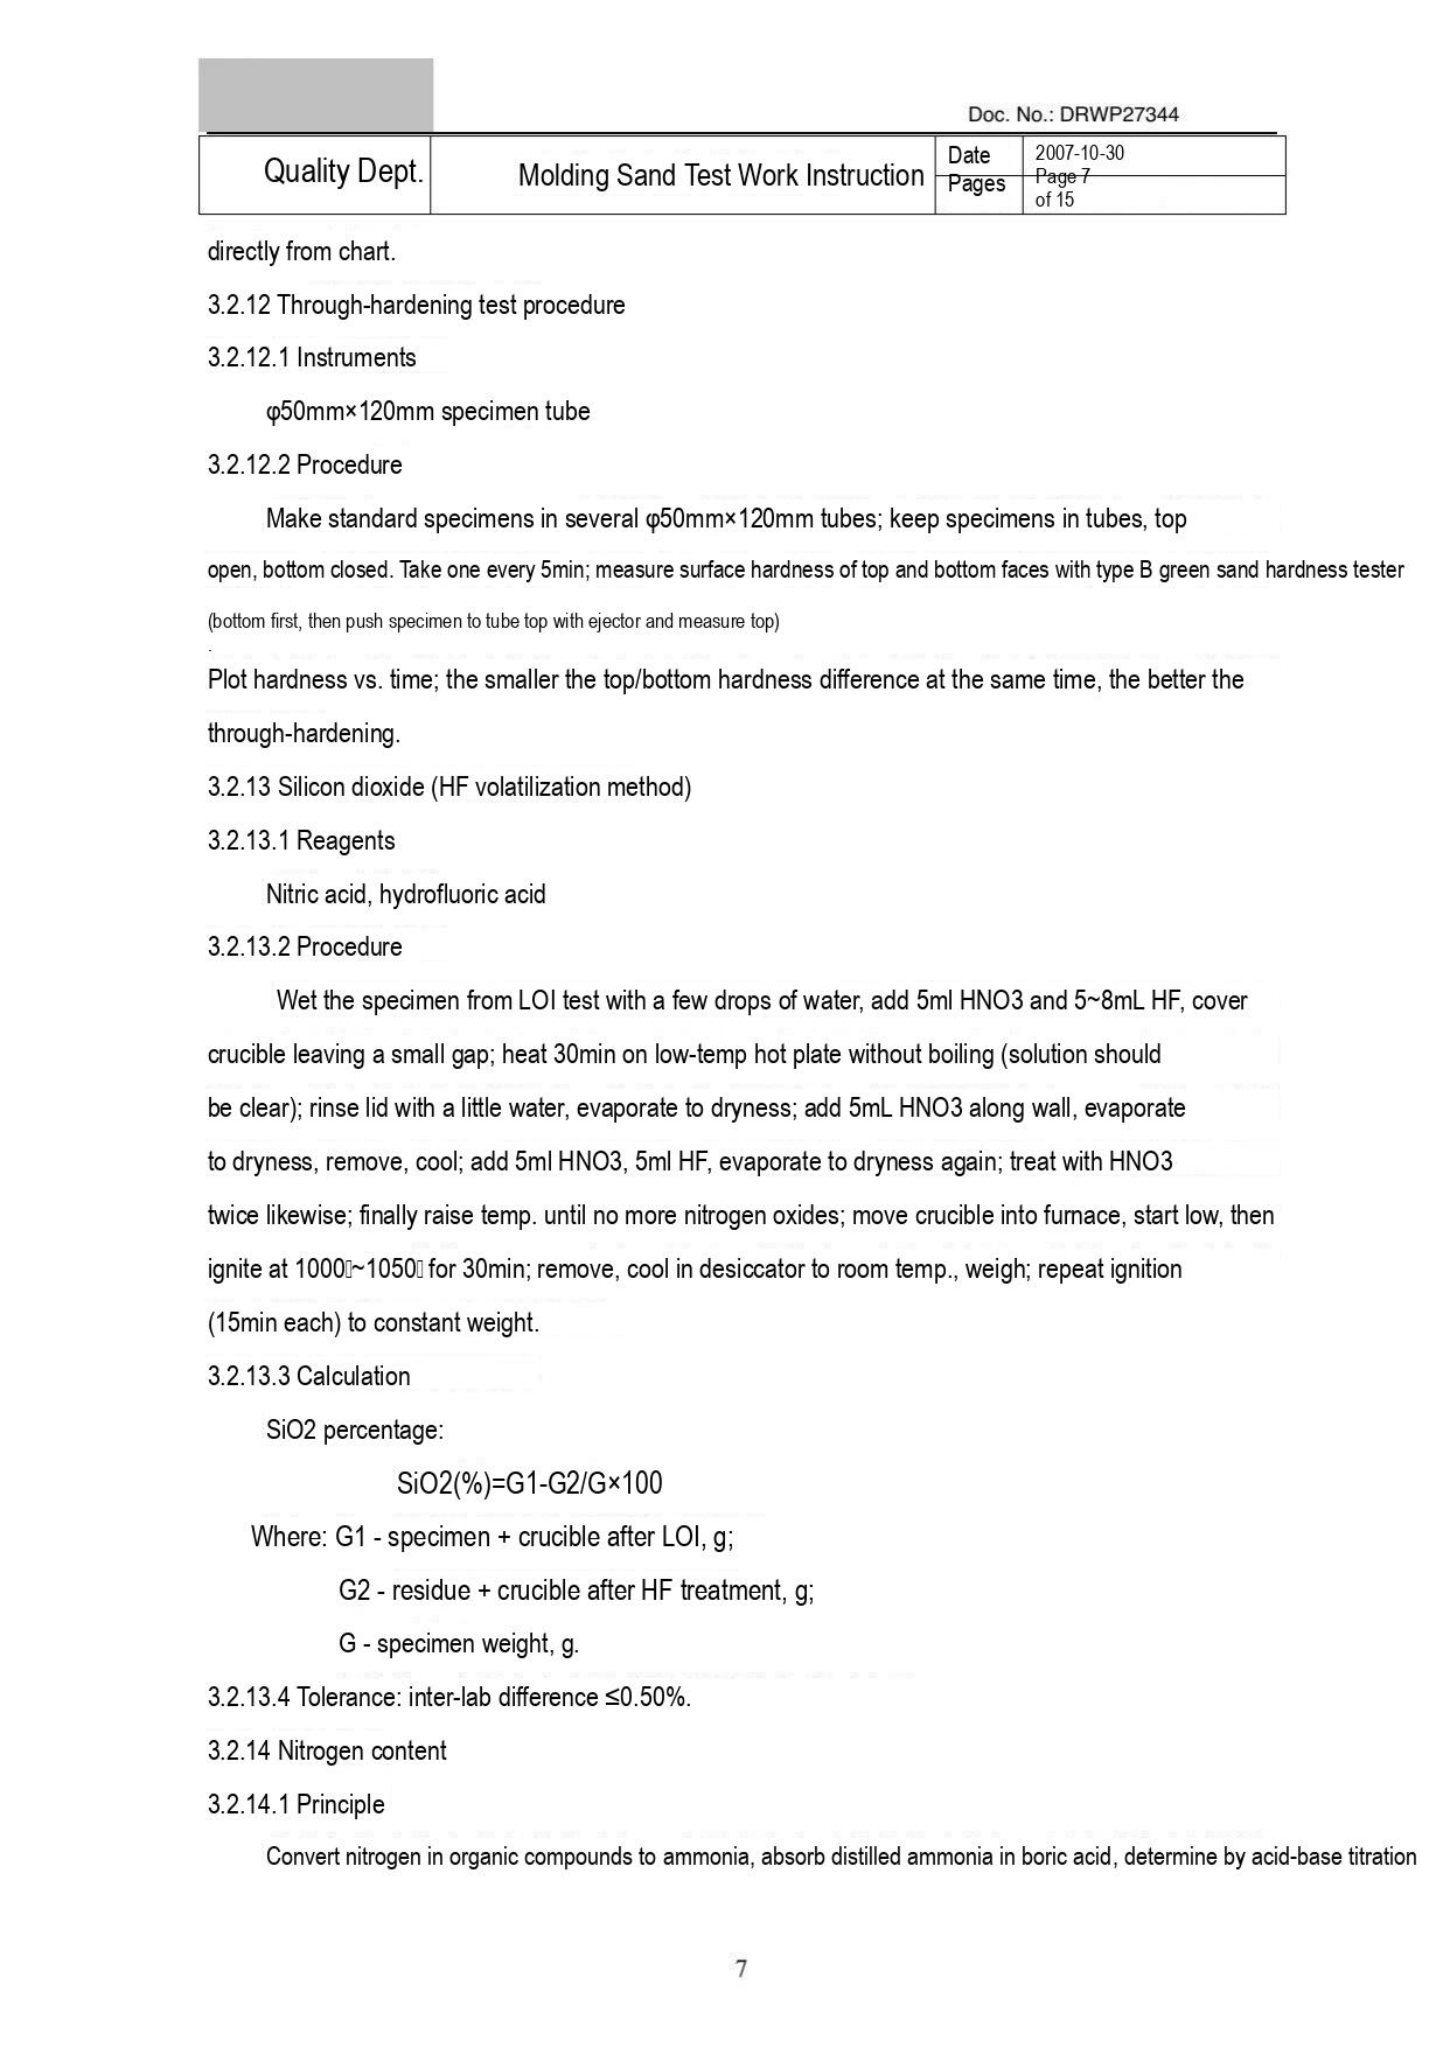Doc. No.: DRWP27344

| Quality Dept. | Molding Sand Test Work Instruction | Date | 2007-10-30 |
|---|---|---|---|
| | | Pages | Page 7 of 15 |

directly from chart.

3.2.12 Through-hardening test procedure

3.2.12.1 Instruments

φ50mm×120mm specimen tube

3.2.12.2 Procedure

Make standard specimens in several φ50mm×120mm tubes; keep specimens in tubes, top open, bottom closed. Take one every 5min; measure surface hardness of top and bottom faces with type B green sand hardness tester (bottom first, then push specimen to tube top with ejector and measure top)

Plot hardness vs. time; the smaller the top/bottom hardness difference at the same time, the better the through-hardening.

3.2.13 Silicon dioxide (HF volatilization method)

3.2.13.1 Reagents

Nitric acid, hydrofluoric acid

3.2.13.2 Procedure

Wet the specimen from LOI test with a few drops of water, add 5ml HNO3 and 5~8mL HF, cover crucible leaving a small gap; heat 30min on low-temp hot plate without boiling (solution should be clear); rinse lid with a little water, evaporate to dryness; add 5mL HNO3 along wall, evaporate to dryness, remove, cool; add 5ml HNO3, 5ml HF, evaporate to dryness again; treat with HNO3 twice likewise; finally raise temp. until no more nitrogen oxides; move crucible into furnace, start low, then ignite at 1000~1050 for 30min; remove, cool in desiccator to room temp., weigh; repeat ignition (15min each) to constant weight.

3.2.13.3 Calculation

SiO2 percentage:

SiO2(%)=G1-G2/G×100

Where: G1 - specimen + crucible after LOI, g;

G2 - residue + crucible after HF treatment, g;

G - specimen weight, g.

3.2.13.4 Tolerance: inter-lab difference ≤0.50%.

3.2.14 Nitrogen content

3.2.14.1 Principle

Convert nitrogen in organic compounds to ammonia, absorb distilled ammonia in boric acid, determine by acid-base titration

7
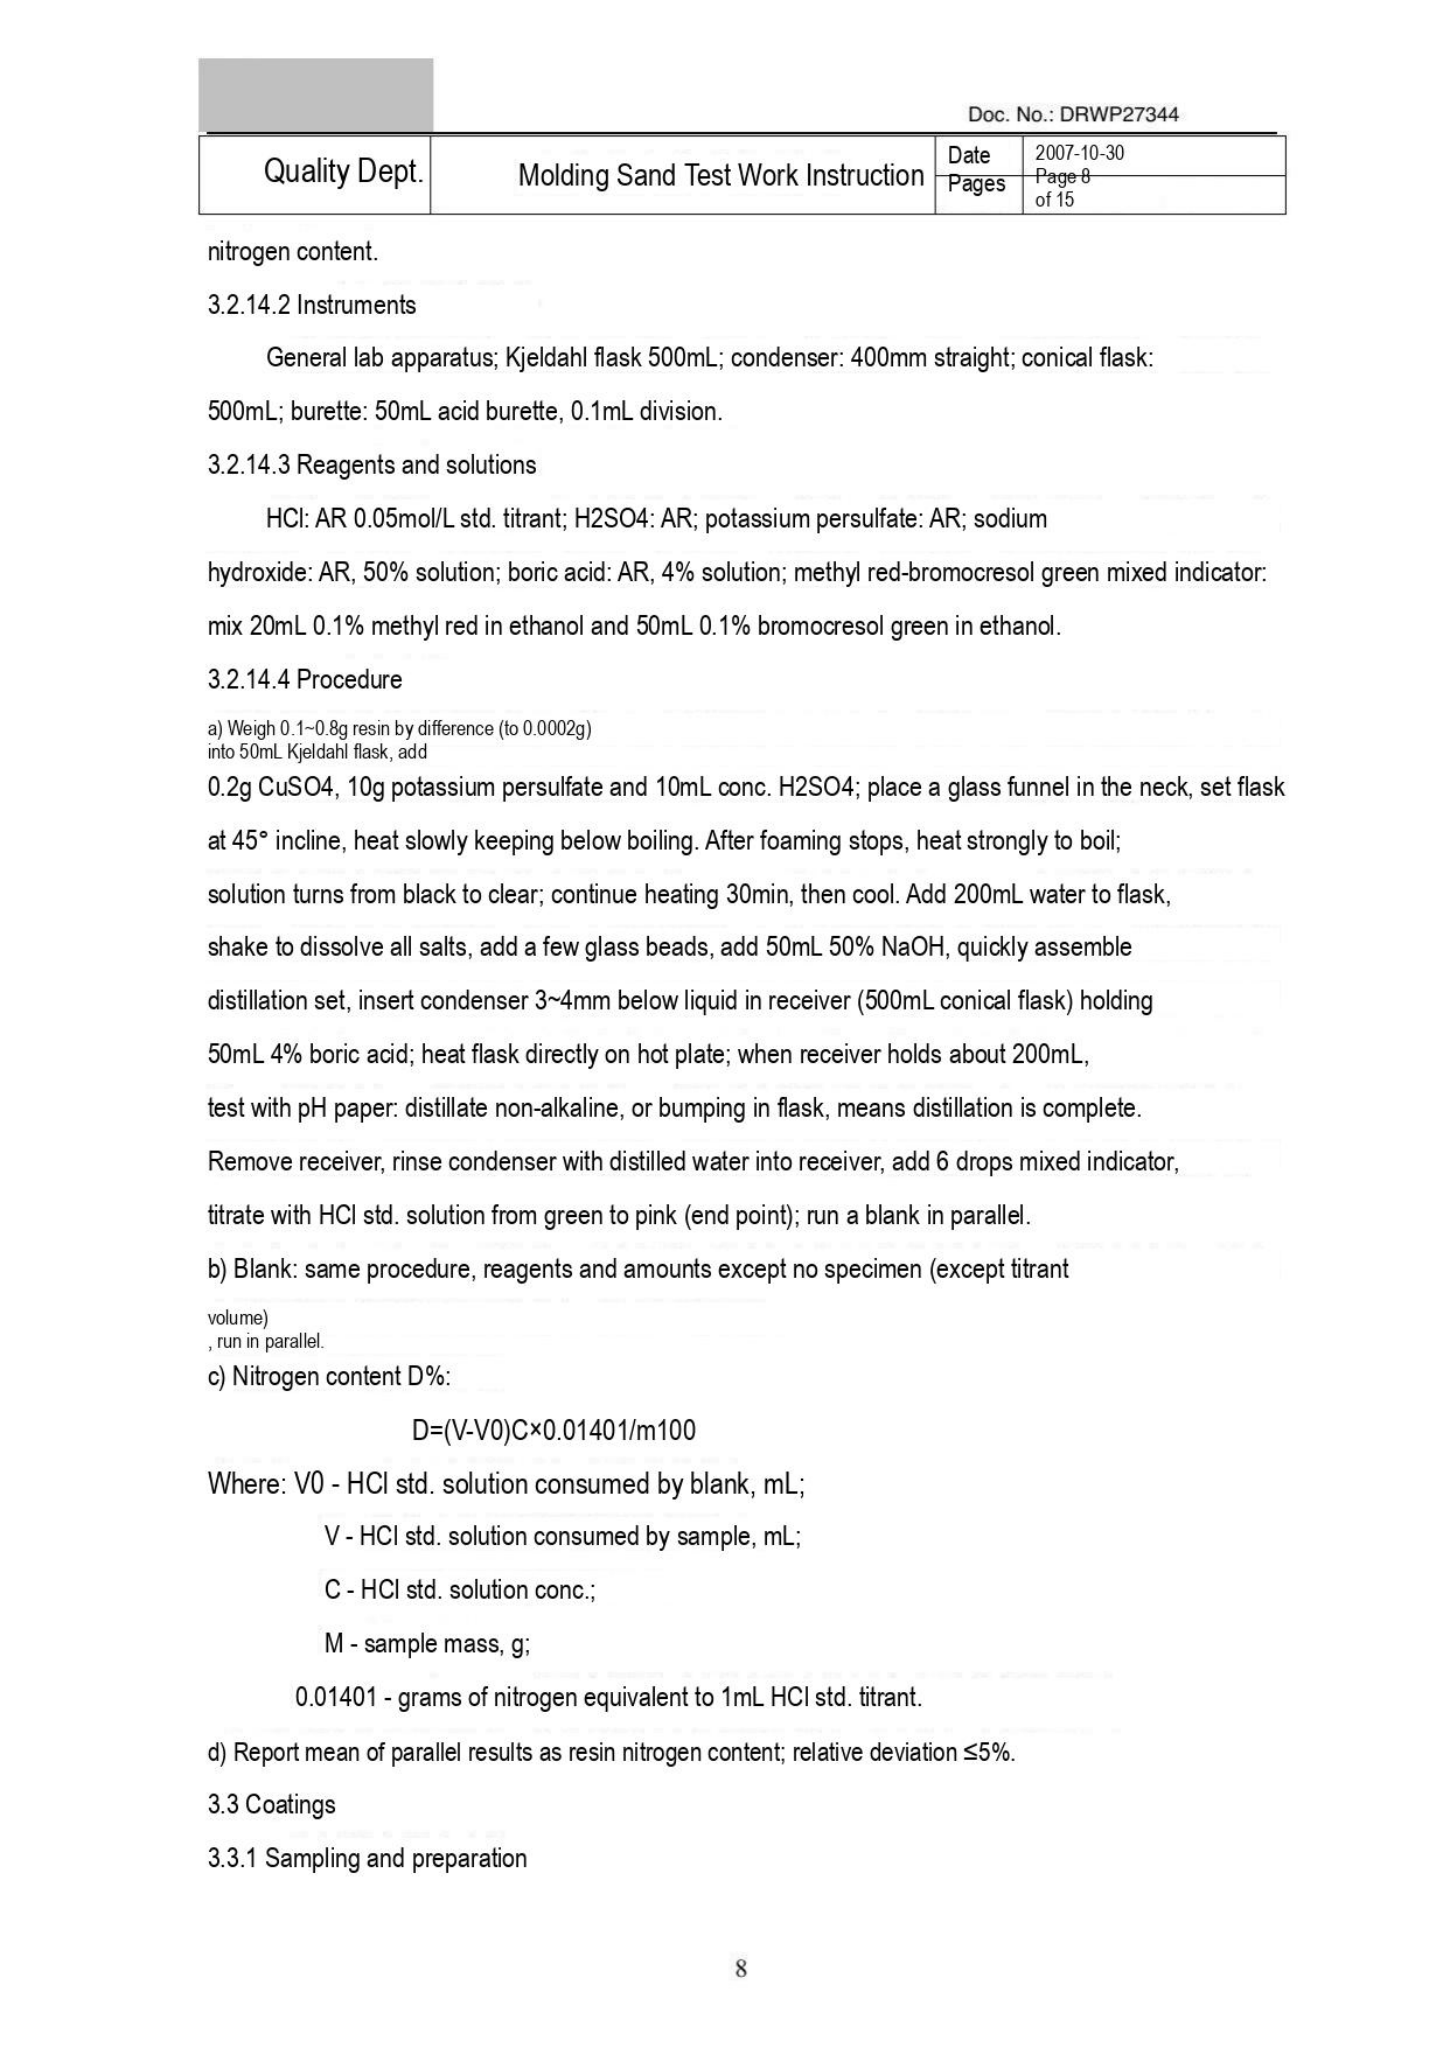Doc. No.: DRWP27344

| Quality Dept. | Molding Sand Test Work Instruction | Date | 2007-10-30 |
|---|---|---|---|
| | | Pages | Page 8 of 15 |

nitrogen content.

3.2.14.2 Instruments

General lab apparatus; Kjeldahl flask 500mL; condenser: 400mm straight; conical flask: 500mL; burette: 50mL acid burette, 0.1mL division.

3.2.14.3 Reagents and solutions

HCl: AR 0.05mol/L std. titrant; H2SO4: AR; potassium persulfate: AR; sodium hydroxide: AR, 50% solution; boric acid: AR, 4% solution; methyl red-bromocresol green mixed indicator: mix 20mL 0.1% methyl red in ethanol and 50mL 0.1% bromocresol green in ethanol.

3.2.14.4 Procedure

a) Weigh 0.1~0.8g resin by difference (to 0.0002g)
into 50mL Kjeldahl flask, add
0.2g CuSO4, 10g potassium persulfate and 10mL conc. H2SO4; place a glass funnel in the neck, set flask at 45° incline, heat slowly keeping below boiling. After foaming stops, heat strongly to boil; solution turns from black to clear; continue heating 30min, then cool. Add 200mL water to flask, shake to dissolve all salts, add a few glass beads, add 50mL 50% NaOH, quickly assemble distillation set, insert condenser 3~4mm below liquid in receiver (500mL conical flask) holding 50mL 4% boric acid; heat flask directly on hot plate; when receiver holds about 200mL, test with pH paper: distillate non-alkaline, or bumping in flask, means distillation is complete. Remove receiver, rinse condenser with distilled water into receiver, add 6 drops mixed indicator, titrate with HCl std. solution from green to pink (end point); run a blank in parallel.

b) Blank: same procedure, reagents and amounts except no specimen (except titrant
volume)
, run in parallel.

c) Nitrogen content D%:

D=(V-V0)C×0.01401/m100

Where: V0 - HCl std. solution consumed by blank, mL;

V - HCl std. solution consumed by sample, mL;

C - HCl std. solution conc.;

M - sample mass, g;

0.01401 - grams of nitrogen equivalent to 1mL HCl std. titrant.

d) Report mean of parallel results as resin nitrogen content; relative deviation ≤5%.

3.3 Coatings

3.3.1 Sampling and preparation

8
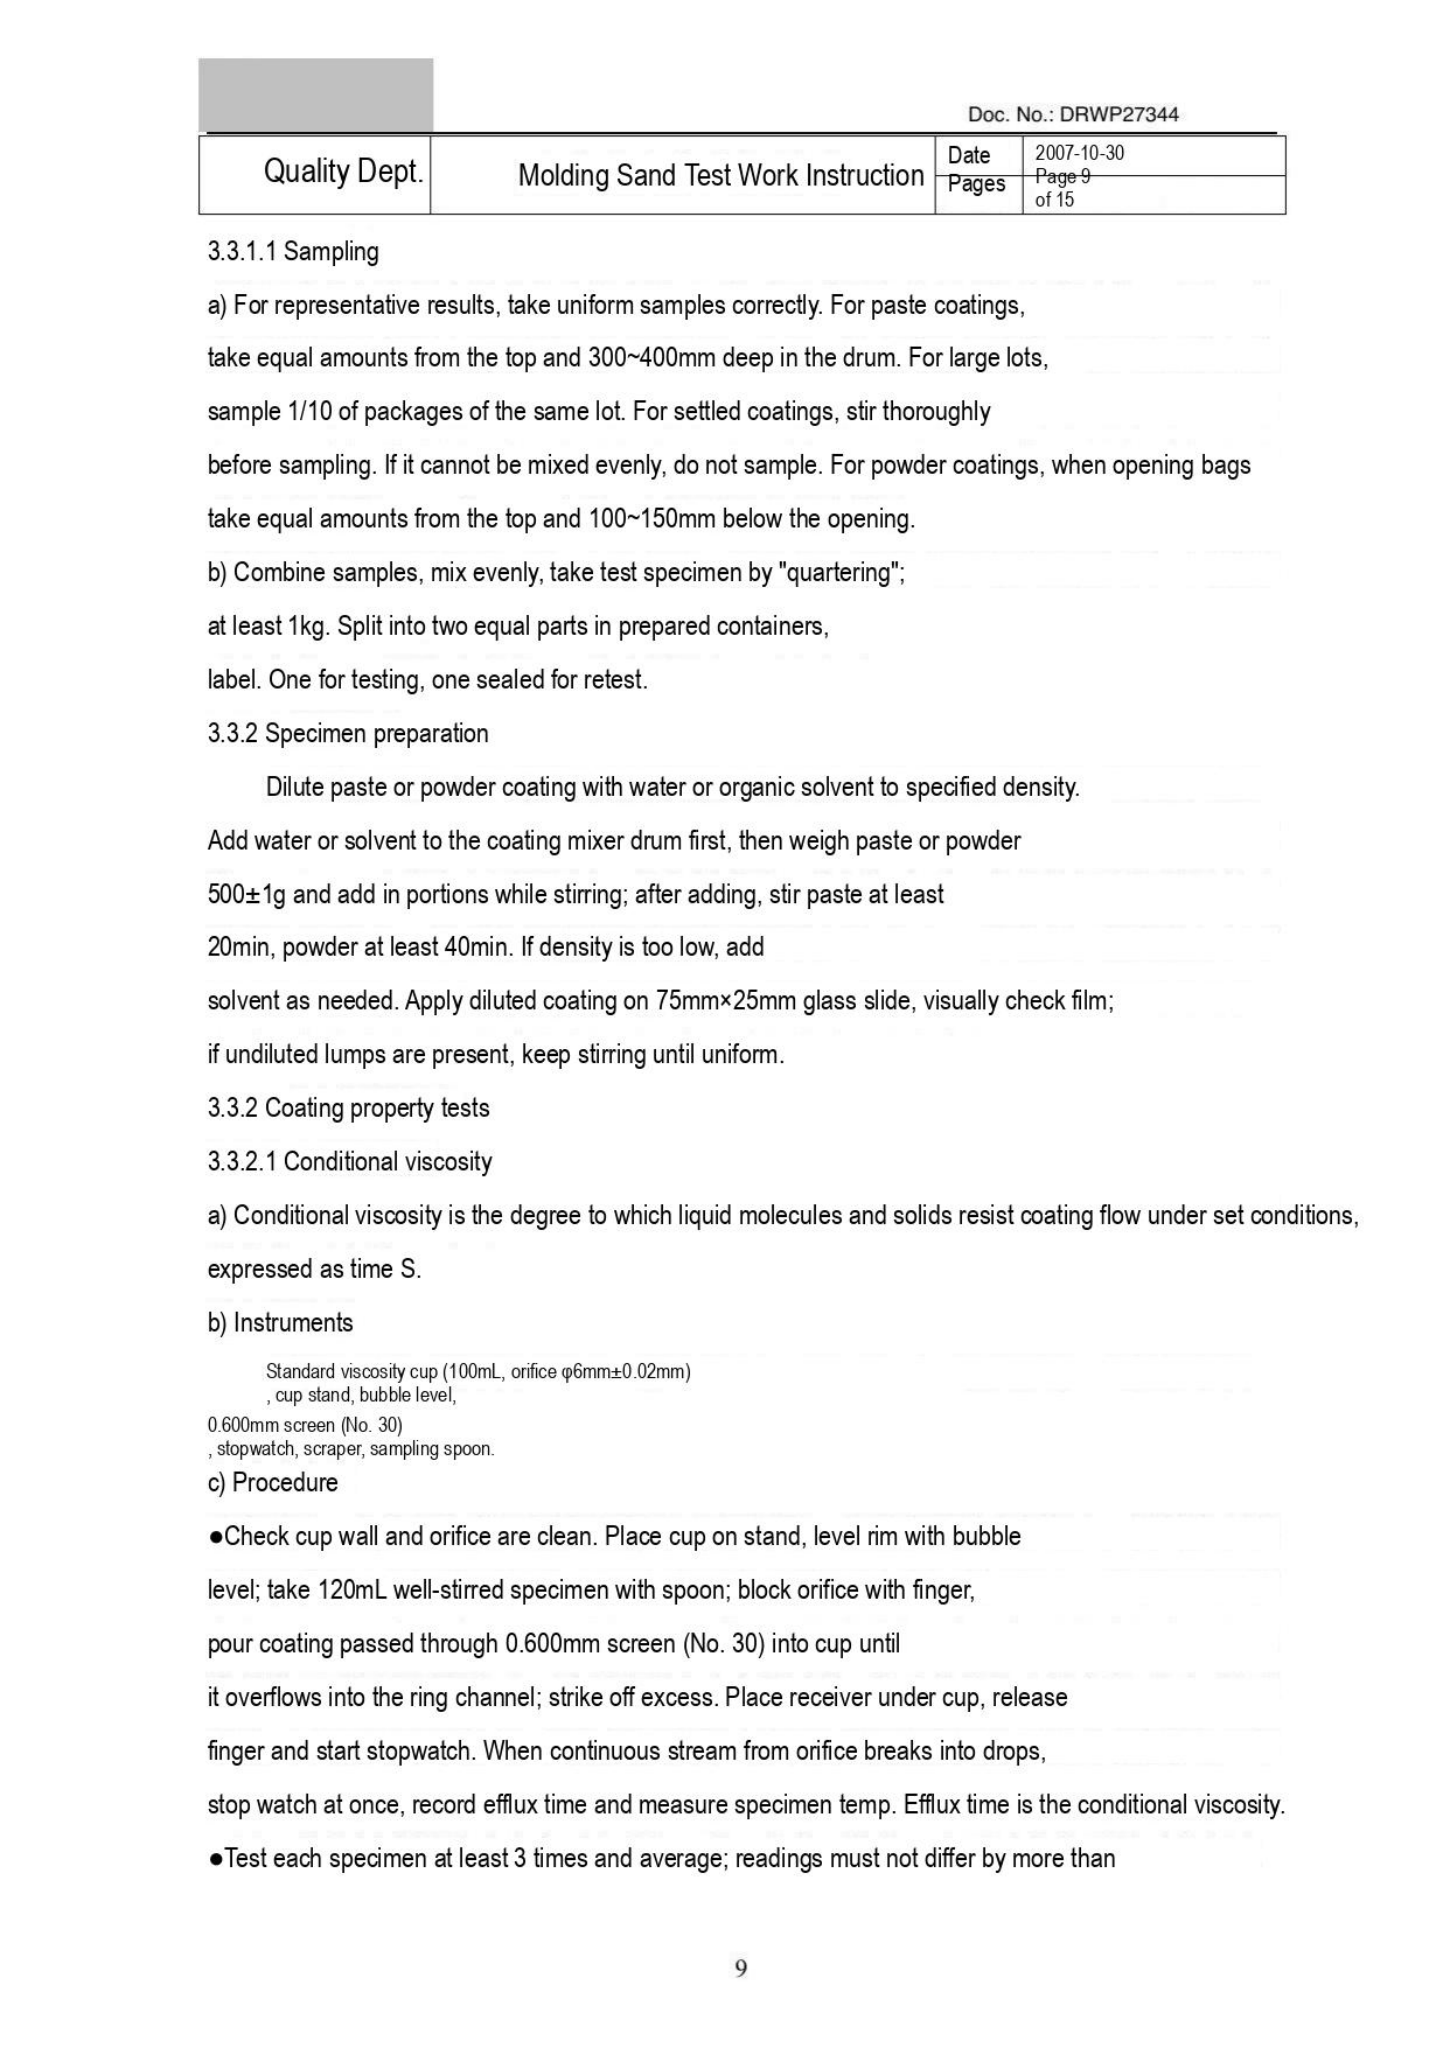Doc. No.: DRWP27344

| Quality Dept. | Molding Sand Test Work Instruction | Date | 2007-10-30 |
|---|---|---|---|
| | | Pages | Page 9 of 15 |

3.3.1.1 Sampling

a) For representative results, take uniform samples correctly. For paste coatings, take equal amounts from the top and 300~400mm deep in the drum. For large lots, sample 1/10 of packages of the same lot. For settled coatings, stir thoroughly before sampling. If it cannot be mixed evenly, do not sample. For powder coatings, when opening bags take equal amounts from the top and 100~150mm below the opening.

b) Combine samples, mix evenly, take test specimen by "quartering"; at least 1kg. Split into two equal parts in prepared containers, label. One for testing, one sealed for retest.

3.3.2 Specimen preparation

Dilute paste or powder coating with water or organic solvent to specified density. Add water or solvent to the coating mixer drum first, then weigh paste or powder 500±1g and add in portions while stirring; after adding, stir paste at least 20min, powder at least 40min. If density is too low, add solvent as needed. Apply diluted coating on 75mm×25mm glass slide, visually check film; if undiluted lumps are present, keep stirring until uniform.

3.3.2 Coating property tests

3.3.2.1 Conditional viscosity

a) Conditional viscosity is the degree to which liquid molecules and solids resist coating flow under set conditions, expressed as time S.

b) Instruments

Standard viscosity cup (100mL, orifice φ6mm±0.02mm)
, cup stand, bubble level,
0.600mm screen (No. 30)
, stopwatch, scraper, sampling spoon.

c) Procedure

●Check cup wall and orifice are clean. Place cup on stand, level rim with bubble level; take 120mL well-stirred specimen with spoon; block orifice with finger, pour coating passed through 0.600mm screen (No. 30) into cup until it overflows into the ring channel; strike off excess. Place receiver under cup, release finger and start stopwatch. When continuous stream from orifice breaks into drops, stop watch at once, record efflux time and measure specimen temp. Efflux time is the conditional viscosity.

●Test each specimen at least 3 times and average; readings must not differ by more than

9
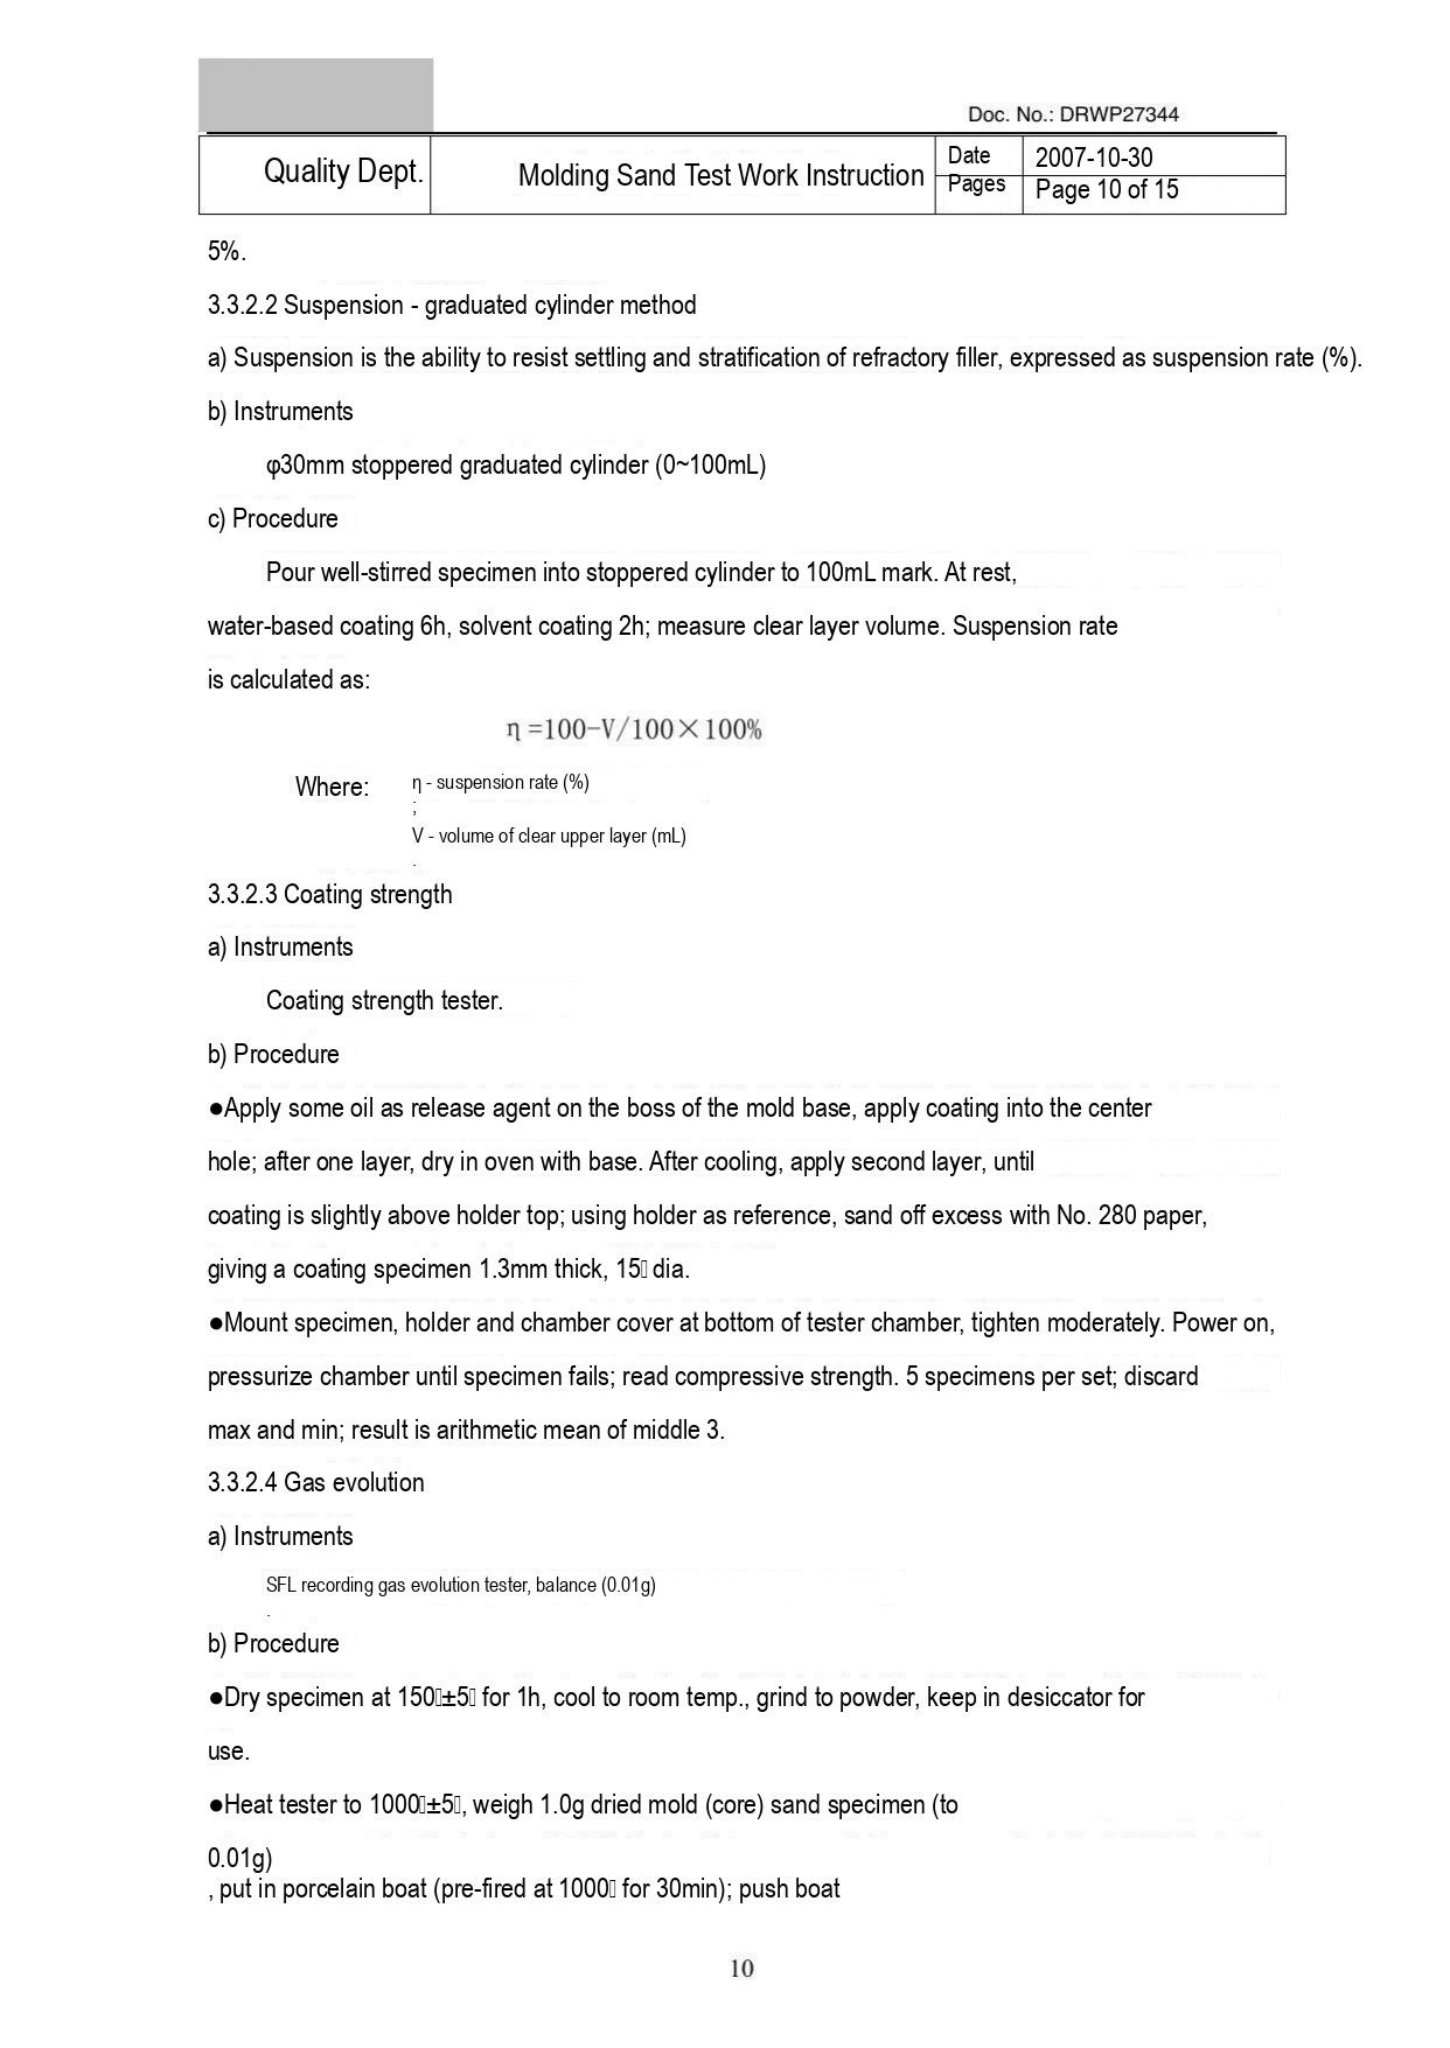Doc. No.: DRWP27344

| Quality Dept. | Molding Sand Test Work Instruction | Date | 2007-10-30 |
|---|---|---|---|
| | | Pages | Page 10 of 15 |

5%.

3.3.2.2 Suspension - graduated cylinder method

a) Suspension is the ability to resist settling and stratification of refractory filler, expressed as suspension rate (%).

b) Instruments

φ30mm stoppered graduated cylinder (0~100mL)

c) Procedure

Pour well-stirred specimen into stoppered cylinder to 100mL mark. At rest, water-based coating 6h, solvent coating 2h; measure clear layer volume. Suspension rate is calculated as:

η =100−V/100×100%

Where: η - suspension rate (%)
;
V - volume of clear upper layer (mL)
.

3.3.2.3 Coating strength

a) Instruments

Coating strength tester.

b) Procedure

●Apply some oil as release agent on the boss of the mold base, apply coating into the center hole; after one layer, dry in oven with base. After cooling, apply second layer, until coating is slightly above holder top; using holder as reference, sand off excess with No. 280 paper, giving a coating specimen 1.3mm thick, 15 dia.

●Mount specimen, holder and chamber cover at bottom of tester chamber, tighten moderately. Power on, pressurize chamber until specimen fails; read compressive strength. 5 specimens per set; discard max and min; result is arithmetic mean of middle 3.

3.3.2.4 Gas evolution

a) Instruments

SFL recording gas evolution tester, balance (0.01g)
.

b) Procedure

●Dry specimen at 150±5 for 1h, cool to room temp., grind to powder, keep in desiccator for use.

●Heat tester to 1000±5, weigh 1.0g dried mold (core) sand specimen (to 0.01g)
, put in porcelain boat (pre-fired at 1000 for 30min); push boat

10
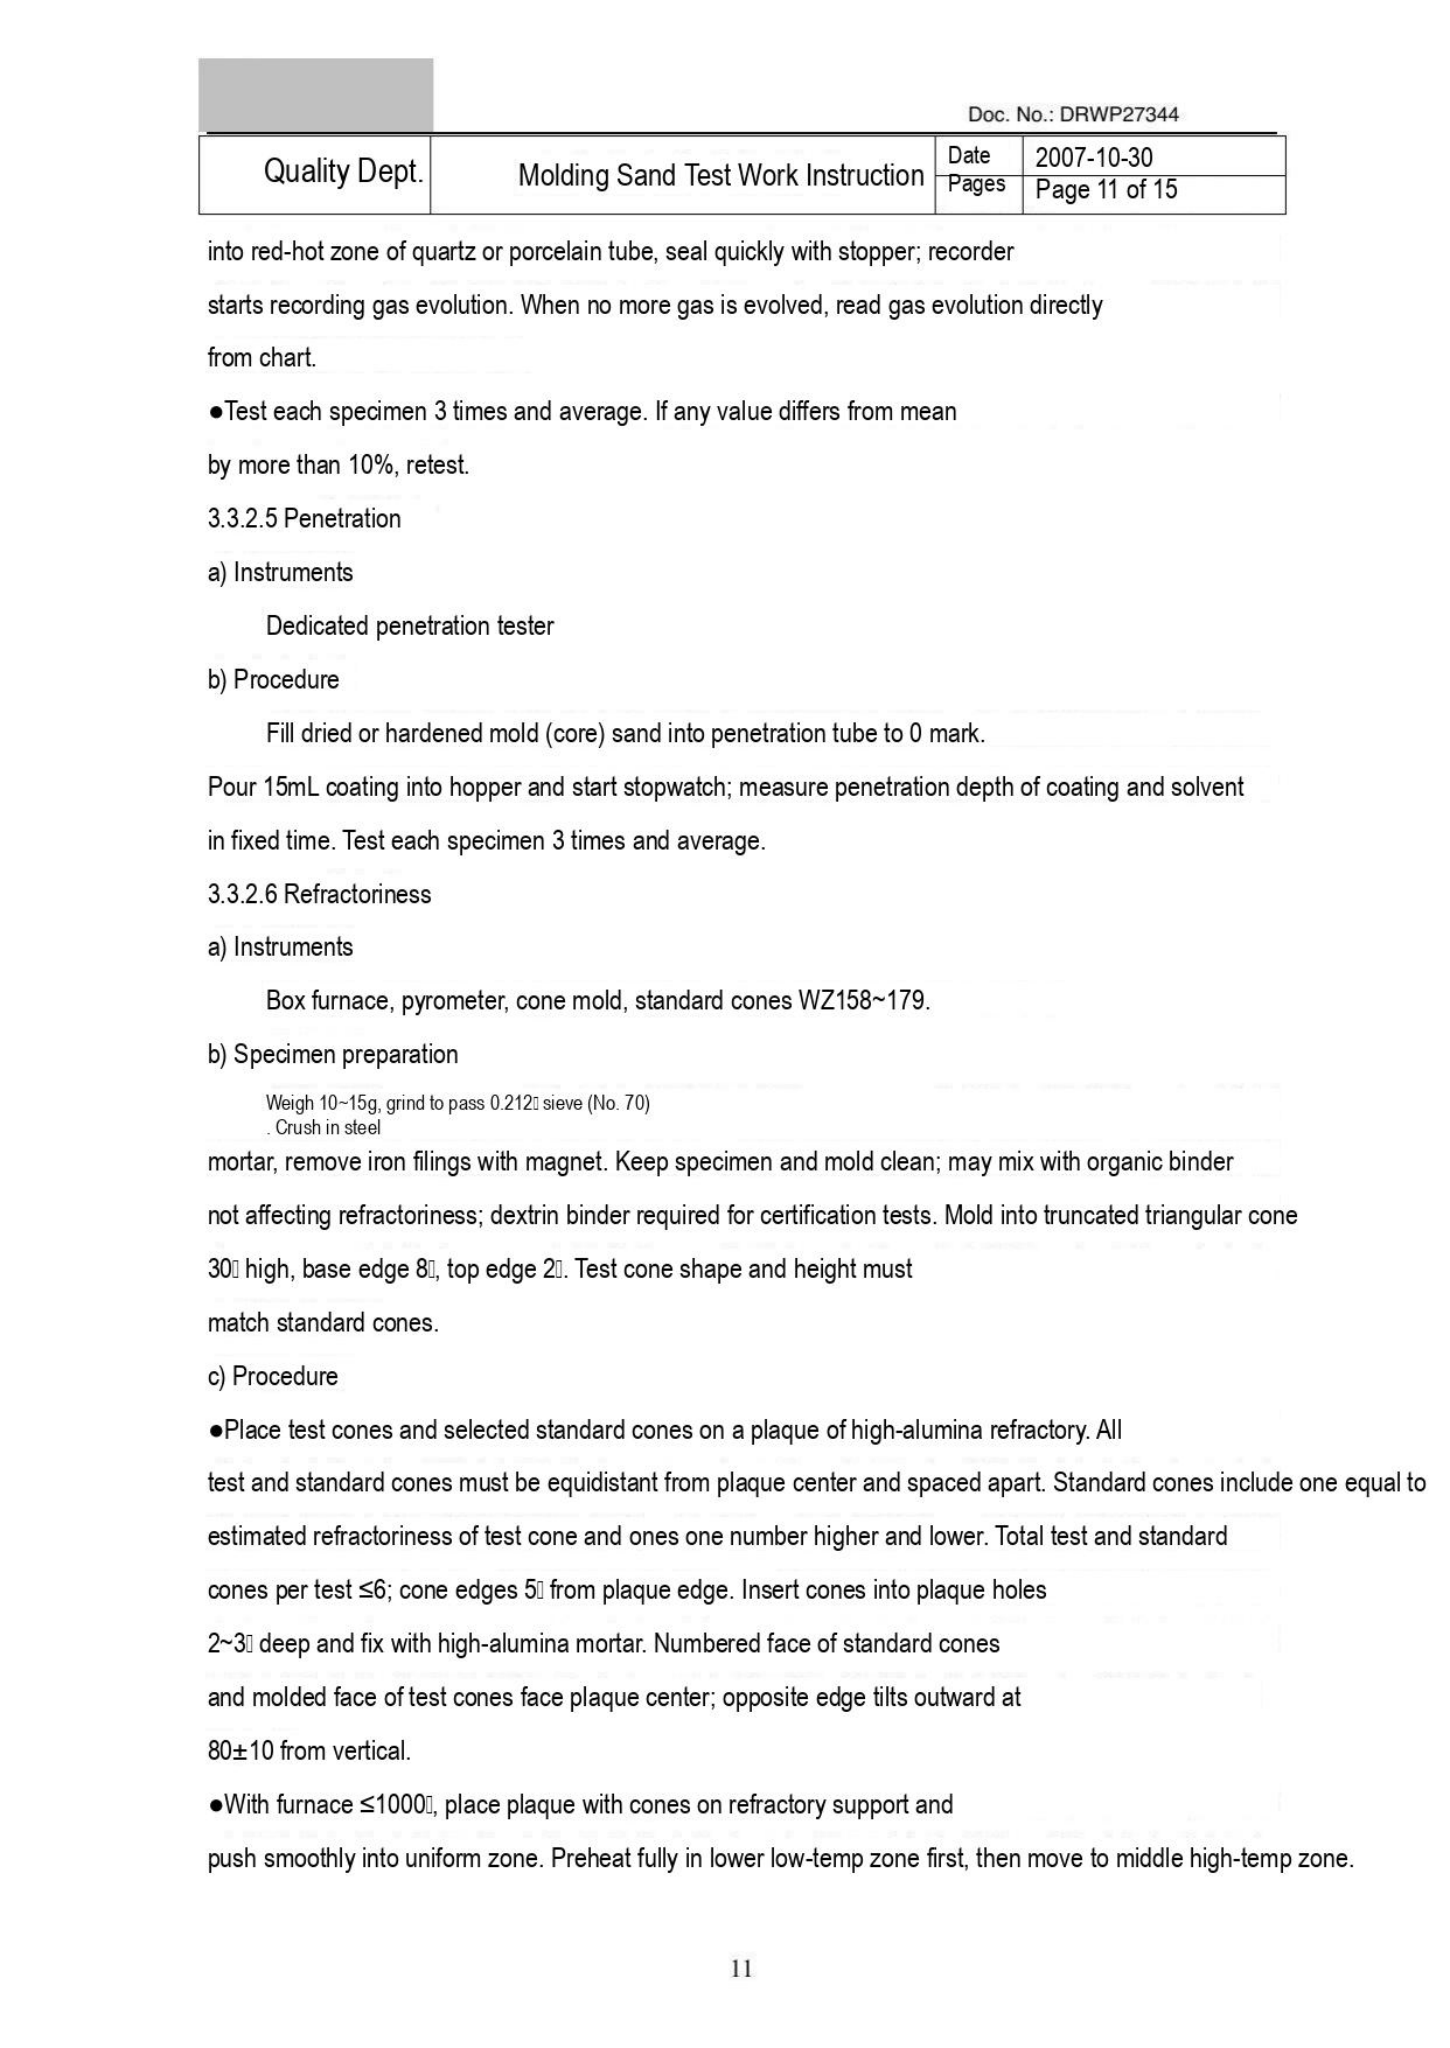Doc. No.: DRWP27344

| Quality Dept. | Molding Sand Test Work Instruction | Date | 2007-10-30 |
|---|---|---|---|
| | | Pages | Page 11 of 15 |

into red-hot zone of quartz or porcelain tube, seal quickly with stopper; recorder

starts recording gas evolution. When no more gas is evolved, read gas evolution directly

from chart.

●Test each specimen 3 times and average. If any value differs from mean

by more than 10%, retest.

3.3.2.5 Penetration

a) Instruments

Dedicated penetration tester

b) Procedure

Fill dried or hardened mold (core) sand into penetration tube to 0 mark.

Pour 15mL coating into hopper and start stopwatch; measure penetration depth of coating and solvent

in fixed time. Test each specimen 3 times and average.

3.3.2.6 Refractoriness

a) Instruments

Box furnace, pyrometer, cone mold, standard cones WZ158~179.

b) Specimen preparation

Weigh 10~15g, grind to pass 0.212 sieve (No. 70)
. Crush in steel

mortar, remove iron filings with magnet. Keep specimen and mold clean; may mix with organic binder

not affecting refractoriness; dextrin binder required for certification tests. Mold into truncated triangular cone

30 high, base edge 8, top edge 2. Test cone shape and height must

match standard cones.

c) Procedure

●Place test cones and selected standard cones on a plaque of high-alumina refractory. All

test and standard cones must be equidistant from plaque center and spaced apart. Standard cones include one equal to

estimated refractoriness of test cone and ones one number higher and lower. Total test and standard

cones per test ≤6; cone edges 5 from plaque edge. Insert cones into plaque holes

2~3 deep and fix with high-alumina mortar. Numbered face of standard cones

and molded face of test cones face plaque center; opposite edge tilts outward at

80±10 from vertical.

●With furnace ≤1000, place plaque with cones on refractory support and

push smoothly into uniform zone. Preheat fully in lower low-temp zone first, then move to middle high-temp zone.

11
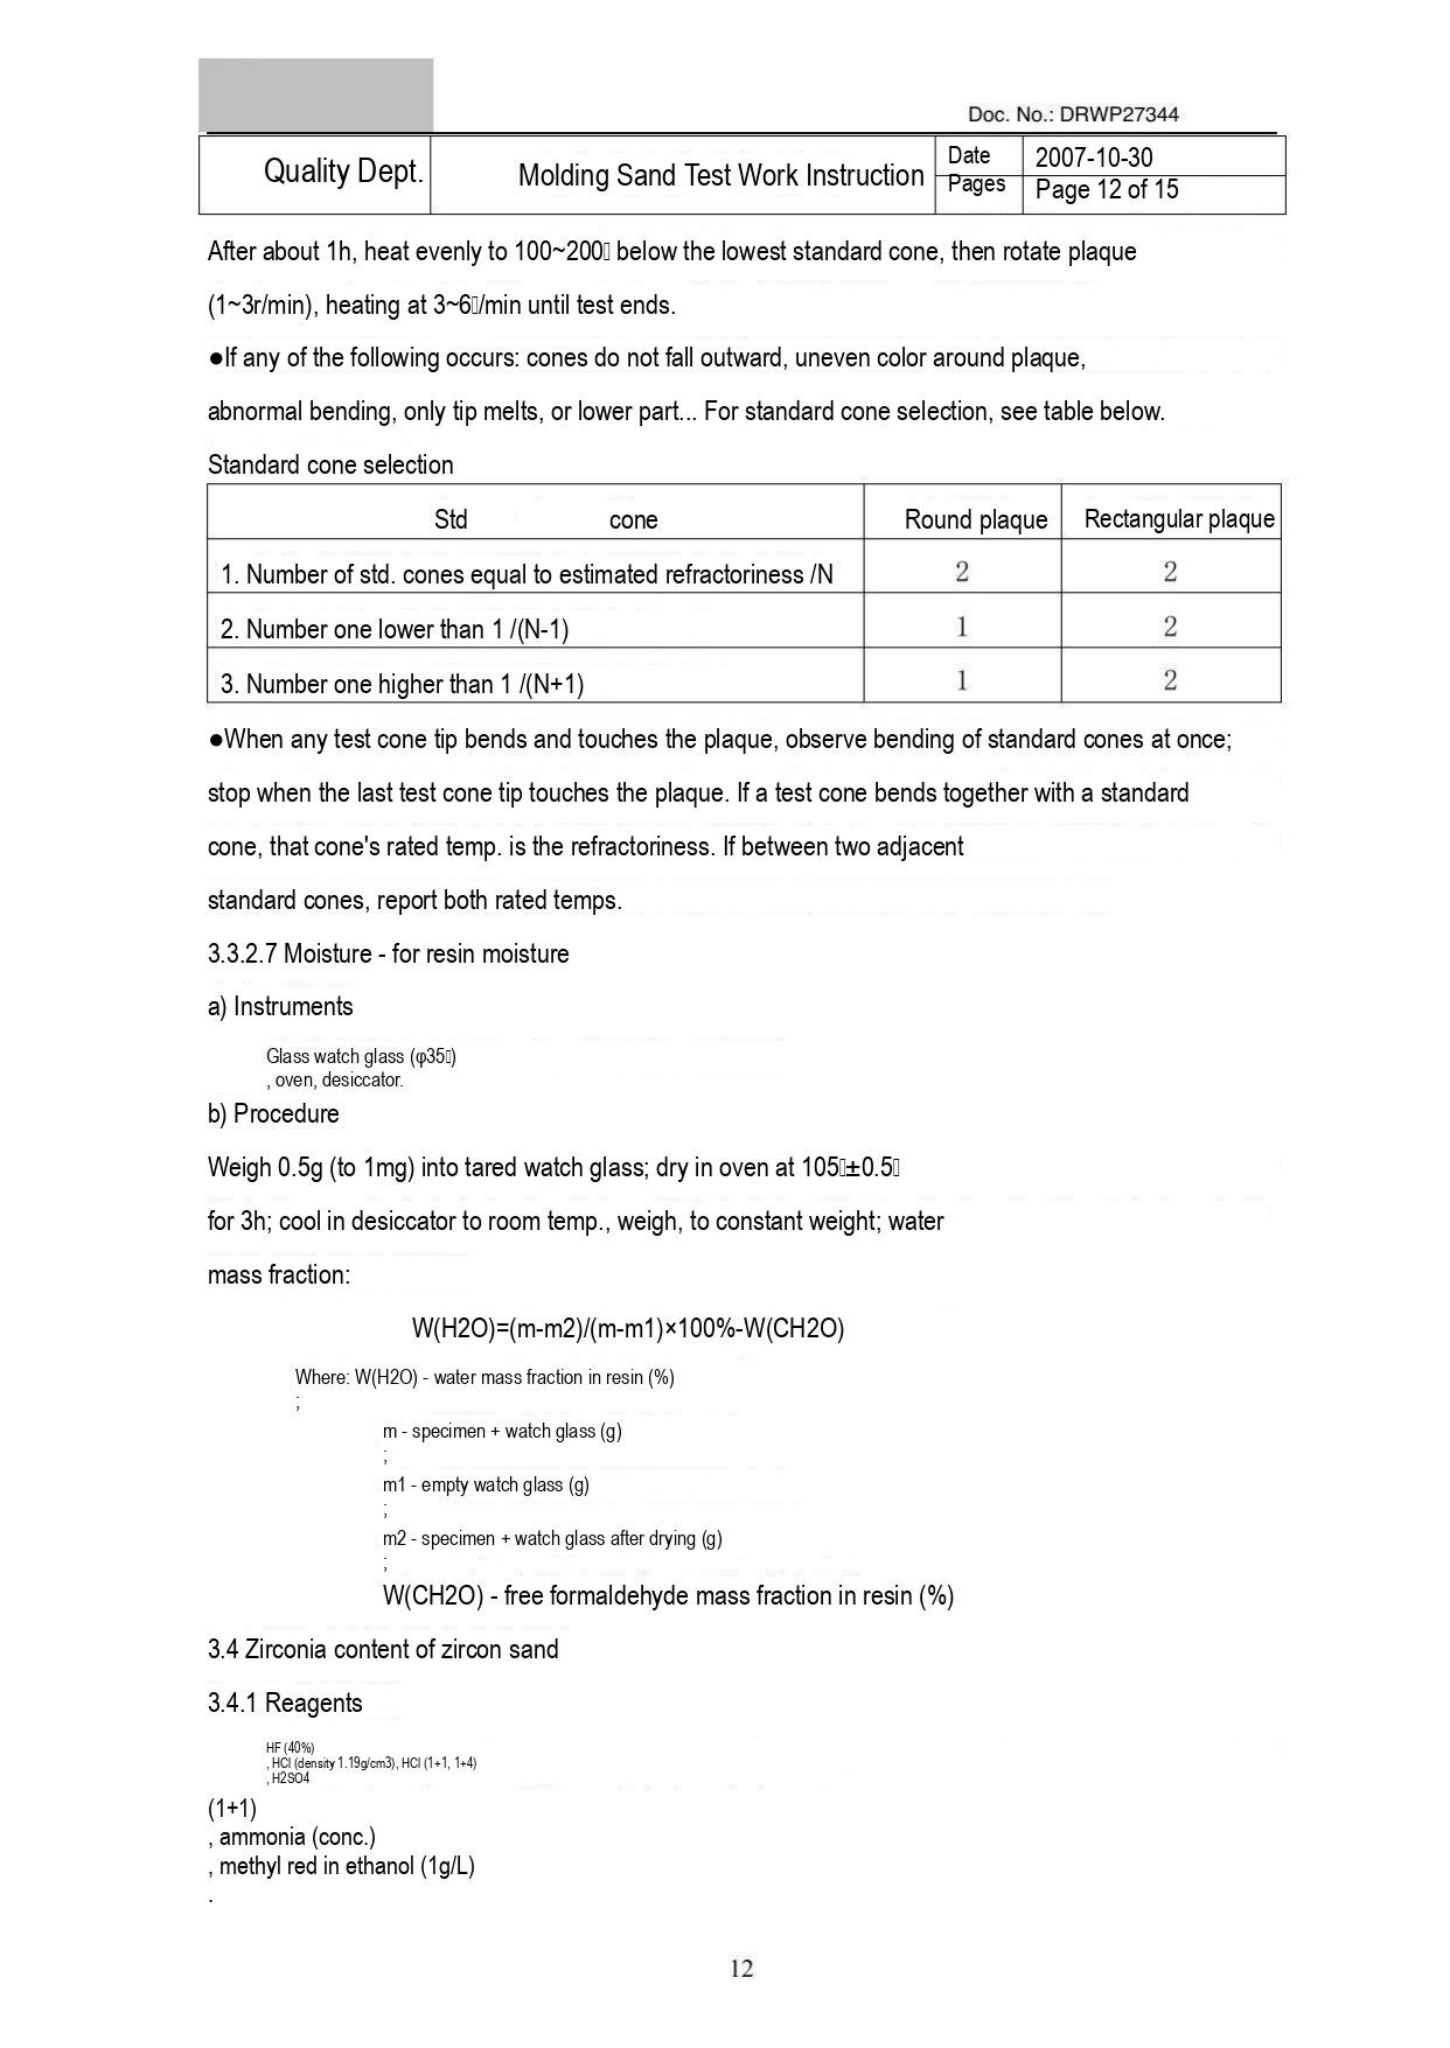Doc. No.: DRWP27344

| Quality Dept. | Molding Sand Test Work Instruction | Date | 2007-10-30 |
|---|---|---|---|
| | | Pages | Page 12 of 15 |

After about 1h, heat evenly to 100~200 below the lowest standard cone, then rotate plaque (1~3r/min), heating at 3~6/min until test ends.

●If any of the following occurs: cones do not fall outward, uneven color around plaque, abnormal bending, only tip melts, or lower part... For standard cone selection, see table below.

Standard cone selection

| Std cone | Round plaque | Rectangular plaque |
|---|---|---|
| 1. Number of std. cones equal to estimated refractoriness /N | 2 | 2 |
| 2. Number one lower than 1 /(N-1) | 1 | 2 |
| 3. Number one higher than 1 /(N+1) | 1 | 2 |

●When any test cone tip bends and touches the plaque, observe bending of standard cones at once; stop when the last test cone tip touches the plaque. If a test cone bends together with a standard cone, that cone's rated temp. is the refractoriness. If between two adjacent standard cones, report both rated temps.

3.3.2.7 Moisture - for resin moisture

a) Instruments

Glass watch glass (φ35)
, oven, desiccator.

b) Procedure

Weigh 0.5g (to 1mg) into tared watch glass; dry in oven at 105±0.5 for 3h; cool in desiccator to room temp., weigh, to constant weight; water mass fraction:

W(H2O)=(m-m2)/(m-m1)×100%-W(CH2O)

Where: W(H2O) - water mass fraction in resin (%)
;

m - specimen + watch glass (g)
;

m1 - empty watch glass (g)
;

m2 - specimen + watch glass after drying (g)
;

W(CH2O) - free formaldehyde mass fraction in resin (%)

3.4 Zirconia content of zircon sand

3.4.1 Reagents

HF (40%)
, HCl (density 1.19g/cm3), HCl (1+1, 1+4)
, H2SO4
(1+1)
, ammonia (conc.)
, methyl red in ethanol (1g/L)
.

12